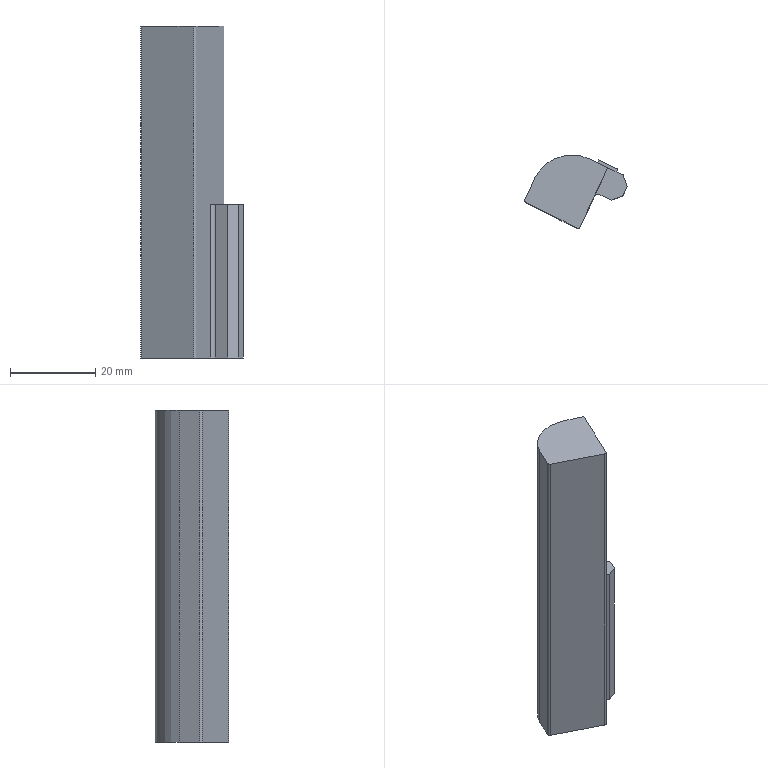Part | STEP file | gslz 2016.10.28-13_id286_x_t | 1 solid | 19 faces | box 24.117 x 17.224 x 78 mm | volume 17489 mm3 | plane 14 | cylinder 4 | other 1 | commonest cylinder face diameters 1 x2 2 x1 19.5 x1